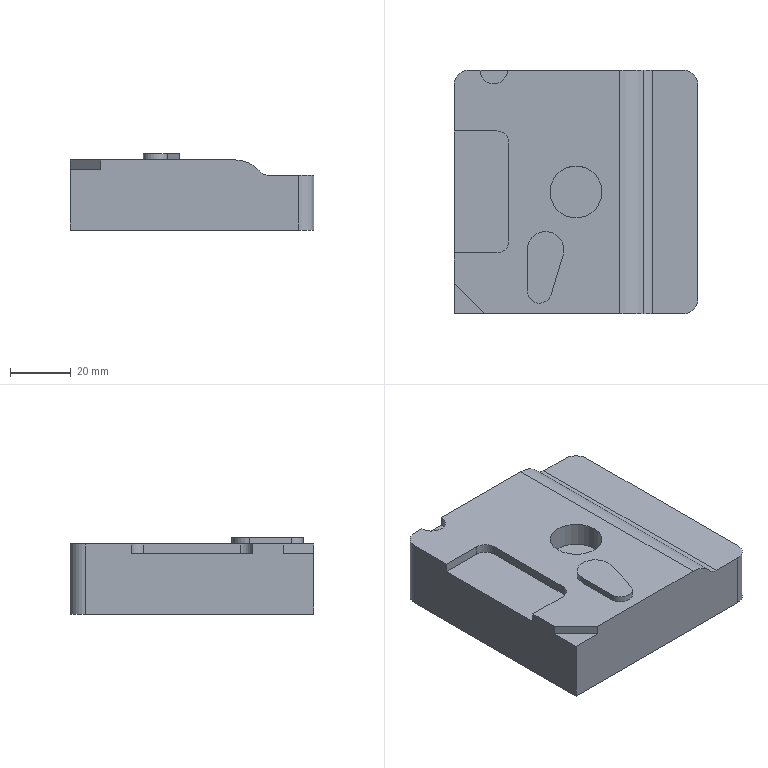NC program | NX | posted with a generic post | part box 80 x 80 x 25 mm
Lines 7698 to 8300 of 8300:
(FIXED_CONTOUR , TOOL : B6)
N15382 M6
N15384 G53
N15386 G17 G0 G90 X25.063 Y43.002 S0 M3
N15388 G43 Z8. H0
N15390 Z-1.995
N15392 G94 G1 Y42.899 Z-2.772 F250.
N15394 Y42.6 Z-3.495
N15396 Y42.123 Z-4.117
N15398 Y41.502 Z-4.594
N15400 Y40.778 Z-4.893
N15402 Y40.002 Z-4.995
N15404 Y38.203
N15406 Y36.403
N15408 Y34.603
N15410 Y32.803
N15412 Y31.003
N15414 Y29.203
N15416 Y27.403
N15418 Y25.603
N15420 Y23.803
N15422 Y22.003
N15424 Y20.203
N15426 Y18.403
N15428 Y16.603
N15430 X25.062 Y14.803
N15432 Y13.003
N15434 Y11.203
N15436 Y9.403
N15438 Y7.603
N15440 Y5.803
N15442 Y4.003
N15444 Y2.203
N15446 Y0.403
N15448 Y-1.397
N15450 Y-3.197
N15452 Y-4.997
N15454 Y-6.797
N15456 Y-8.597
N15458 Y-10.397
N15460 Y-12.197
N15462 Y-13.997
N15464 Y-15.797
N15466 Y-17.597
N15468 Y-19.397
N15470 Y-21.197
N15472 Y-22.997
N15474 Y-24.797
N15476 Y-26.597
N15478 Y-28.397
N15480 Y-30.197
N15482 Y-31.997
N15484 Y-33.797
N15486 Y-35.597
N15488 Y-37.397
N15490 Y-39.197
N15492 Y-40.06 Z-4.996
N15494 X25.026 Y-39.998 Z-4.993
N15496 X24.902 Z-4.981
N15498 X24.736 Z-4.94
N15500 X24.405 Z-4.744
N15502 X24.163 Z-4.49
N15504 Y-39.197
N15506 Y-37.397
N15508 Y-35.597
N15510 Y-33.797
N15512 Y-31.997
N15514 Y-30.197 Z-4.491
N15516 Y-28.397
N15518 Y-26.597
N15520 Y-24.797
N15522 Y-22.997
N15524 Y-21.197
N15526 Y-19.397
N15528 Y-17.597
N15530 Y-15.797
N15532 Y-13.997
N15534 Y-12.197
N15536 Y-10.397
N15538 Y-8.597
N15540 Y-6.797
N15542 Y-4.997
N15544 Y-3.197
N15546 Y-1.397
N15548 Y0.403
N15550 Y2.203
N15552 Y4.003
N15554 Y5.803
N15556 Y7.603
N15558 Y9.403
N15560 Y11.203
N15562 Y13.003
N15564 Y14.803
N15566 X24.164 Y16.603
N15568 Y18.403
N15570 Y20.203
N15572 Y22.003
N15574 Y23.803
N15576 Y25.603
N15578 Y27.403
N15580 Y29.203
N15582 Y31.003
N15584 Y32.803
N15586 Y34.603
N15588 Y36.403
N15590 Y38.203 Z-4.492
N15592 Y39.998
N15594 X23.181 Z-3.476
N15596 Y38.203
N15598 Y36.403
N15600 Y34.603
N15602 Y32.803
N15604 Y31.003
N15606 Y29.203
N15608 Y27.403
N15610 Y25.603
N15612 Y23.803
N15614 Y22.003
N15616 Y20.203
N15618 Y18.403
N15620 Y16.603
N15622 Y14.803
N15624 Y13.003
N15626 Y11.203
N15628 Y9.403
N15630 Y7.603
N15632 Y5.803
N15634 Y4.003
N15636 Y2.203
N15638 Y0.403
N15640 Y-1.397
N15642 Y-3.197
N15644 Y-4.997
N15646 Y-6.797
N15648 Y-8.597
N15650 Y-10.397
N15652 Y-12.197
N15654 Y-13.997
N15656 Y-15.797
N15658 Y-17.597
N15660 Y-19.397
N15662 Y-21.197
N15664 Y-22.997
N15666 Y-24.797
N15668 X23.18 Y-26.597
N15670 Y-28.397
N15672 Y-30.197
N15674 Y-31.997
N15676 Y-33.797
N15678 Y-35.597
N15680 Y-37.397 Z-3.475
N15682 Y-39.197
N15684 Y-39.998
N15686 X22.198 Y-39.992 Z-2.644
N15688 Y-39.197
N15690 Y-37.397
N15692 Y-35.597
N15694 Y-33.797
N15696 Y-31.997
N15698 Y-30.197 Z-2.645
N15700 Y-28.397
N15702 Y-26.597
N15704 Y-24.797
N15706 Y-22.997
N15708 Y-21.197
N15710 Y-19.397
N15712 Y-17.597
N15714 Y-15.797
N15716 Y-13.997
N15718 Y-12.197
N15720 Y-10.397
N15722 Y-8.597
N15724 Y-6.797
N15726 Y-4.997
N15728 Y-3.197
N15730 Y-1.397
N15732 Y0.403
N15734 Y2.203
N15736 Y4.003
N15738 Y5.803
N15740 Y7.603
N15742 Y9.403
N15744 X22.199 Y11.203
N15746 Y13.003
N15748 Y14.803
N15750 Y16.603
N15752 Y18.403
N15754 Y20.203
N15756 Y22.003
N15758 Y23.803
N15760 Y25.603
N15762 Y27.403
N15764 Y29.203
N15766 Y31.003
N15768 Y32.803
N15770 Y34.603
N15772 Y36.403
N15774 Y38.203
N15776 Y39.992
N15778 X21.216 Y39.998 Z-1.974
N15780 Y38.203
N15782 Y36.403
N15784 Y34.603
N15786 Y32.803
N15788 Y31.003
N15790 Y29.203
N15792 Y27.403
N15794 Y25.603
N15796 Y23.803
N15798 Y22.003
N15800 Y20.203
N15802 Y18.403
N15804 Y16.603
N15806 Y14.803
N15808 Y13.003
N15810 Y11.203
N15812 Y9.403
N15814 Y7.603
N15816 Y5.803
N15818 Y4.003
N15820 Y2.203
N15822 Y0.403
N15824 Y-1.397
N15826 Y-3.197
N15828 Y-4.997
N15830 Y-6.797
N15832 Y-8.597
N15834 Y-10.397
N15836 Y-12.197
N15838 Y-13.997
N15840 Y-15.797
N15842 Y-17.597
N15844 Y-19.397
N15846 Y-21.197
N15848 Y-22.997
N15850 Y-24.797
N15852 Y-26.597
N15854 Y-28.397
N15856 Y-30.197
N15858 X21.215 Y-31.997
N15860 Y-33.797
N15862 Y-35.597
N15864 Y-37.397
N15866 Y-39.197
N15868 Y-39.998
N15870 X20.233 Y-39.996 Z-1.42
N15872 Y-39.197
N15874 Y-37.397
N15876 Y-35.597
N15878 Y-33.797
N15880 Y-31.997
N15882 Y-30.197
N15884 Y-28.397
N15886 Y-26.597
N15888 Y-24.797
N15890 Y-22.997
N15892 Y-21.197
N15894 Y-19.397
N15896 Y-17.597
N15898 Y-15.797
N15900 Y-13.997
N15902 Y-12.197
N15904 Y-10.397
N15906 Y-8.597
N15908 Y-6.797
N15910 Y-4.997
N15912 Y-3.197
N15914 Y-1.397
N15916 Y0.403
N15918 Y2.203
N15920 X20.234 Y4.003
N15922 Y5.803
N15924 Y7.603
N15926 Y9.403
N15928 Y11.203
N15930 Y13.003
N15932 Y14.803
N15934 Y16.603
N15936 Y18.403
N15938 Y20.203
N15940 Y22.003
N15942 Y23.803
N15944 Y25.603
N15946 Y27.403
N15948 Y29.203
N15950 Y31.003
N15952 Y32.803
N15954 Y34.603
N15956 Y36.403
N15958 Y38.203
N15960 Y39.996
N15962 X19.252 Y39.991 Z-0.97
N15964 X19.251 Y38.203
N15966 Y36.403
N15968 Y34.603
N15970 Y32.803
N15972 Y31.003
N15974 Y29.203
N15976 Y27.403
N15978 Y25.603
N15980 Y23.803 Z-0.969
N15982 Y22.003
N15984 Y20.203
N15986 Y18.403
N15988 Y16.603
N15990 Y14.803
N15992 Y13.003
N15994 Y11.203
N15996 Y9.403
N15998 Y7.603
N16000 Y5.803
N16002 Y4.003
N16004 Y2.203
N16006 Y0.403
N16008 Y-1.397
N16010 Y-3.197
N16012 Y-4.997
N16014 Y-6.797
N16016 Y-8.597
N16018 Y-10.397
N16020 Y-12.197
N16022 Y-13.997
N16024 Y-15.797
N16026 Y-17.597
N16028 Y-19.397
N16030 Y-21.197
N16032 Y-22.997
N16034 Y-24.797
N16036 Y-26.597
N16038 Y-28.397
N16040 Y-30.197
N16042 Y-31.997
N16044 Y-33.797
N16046 Y-35.597
N16048 X19.25 Y-37.397
N16050 Y-39.197
N16052 Y-39.991
N16054 X18.548 Y-39.998 Z-0.707
N16056 X18.268 Y-39.995 Z-0.612
N16058 Y-39.197
N16060 Y-37.397
N16062 Y-35.597
N16064 Y-33.797
N16066 Y-31.997
N16068 Y-30.197
N16070 Y-28.397
N16072 Y-26.597
N16074 Y-24.797
N16076 Y-22.997
N16078 Y-21.197
N16080 Y-19.397
N16082 Y-17.597
N16084 Y-15.797
N16086 Y-13.997
N16088 Y-12.197
N16090 Y-10.397
N16092 Y-8.597
N16094 Y-6.797
N16096 Y-4.997
N16098 Y-3.197
N16100 X18.269 Y-1.397
N16102 Y0.403
N16104 Y2.203
N16106 Y4.003
N16108 Y5.803
N16110 Y7.603
N16112 Y9.403
N16114 Y11.203
N16116 Y13.003
N16118 Y14.803
N16120 Y16.603
N16122 Y18.403
N16124 Y20.203
N16126 Y22.003
N16128 Y23.803
N16130 Y25.603
N16132 Y27.403
N16134 Y29.203
N16136 Y31.003
N16138 Y32.803
N16140 Y34.603
N16142 Y36.403
N16144 Y38.203
N16146 Y39.995
N16148 X17.806 Y39.991 Z-0.476
N16150 X17.287 Y39.996 Z-0.341
N16152 Y38.203
N16154 Y36.403
N16156 Y34.603
N16158 X17.286 Y32.803
N16160 Y31.003
N16162 Y29.203
N16164 Y27.403
N16166 Y25.603
N16168 Y23.803
N16170 Y22.003
N16172 Y20.203
N16174 Y18.403
N16176 Y16.603
N16178 Y14.803
N16180 Y13.003
N16182 Y11.203
N16184 Y9.403
N16186 Y7.603
N16188 Y5.803
N16190 Y4.003
N16192 Y2.203
N16194 Y0.403
N16196 Y-1.397
N16198 Y-3.197
N16200 Y-4.997
N16202 Y-6.797
N16204 Y-8.597
N16206 Y-10.397
N16208 Y-12.197
N16210 Y-13.997 Z-0.34
N16212 Y-15.797
N16214 Y-17.597
N16216 Y-19.397
N16218 Y-21.197
N16220 Y-22.997
N16222 Y-24.797
N16224 Y-26.597
N16226 Y-28.397
N16228 Y-30.197
N16230 Y-31.997
N16232 Y-33.797
N16234 Y-35.597
N16236 Y-37.397
N16238 Y-39.197
N16240 Y-39.996
N16242 X16.303 Y-39.991 Z-0.15
N16244 Y-39.197
N16246 Y-37.397
N16248 Y-35.597
N16250 Y-33.797
N16252 Y-31.997
N16254 Y-30.197
N16256 Y-28.397
N16258 Y-26.597
N16260 Y-24.797
N16262 Y-22.997
N16264 Y-21.197
N16266 Y-19.397
N16268 Y-17.597
N16270 Y-15.797
N16272 Y-13.997
N16274 Y-12.197
N16276 Y-10.397
N16278 Y-8.597
N16280 X16.304 Y-6.797
N16282 Y-4.997
N16284 Y-3.197
N16286 Y-1.397
N16288 Y0.403
N16290 Y2.203
N16292 Y4.003
N16294 Y5.803
N16296 Y7.603
N16298 Y9.403
N16300 Y11.203
N16302 Y13.003
N16304 Y14.803
N16306 Y16.603
N16308 Y18.403
N16310 Y20.203
N16312 Y22.003
N16314 Y23.803
N16316 Y25.603
N16318 Y27.403
N16320 Y29.203
N16322 Y31.003
N16324 Y32.803
N16326 Y34.603
N16328 Y36.403
N16330 Y38.203
N16332 Y39.991
N16334 X15.322 Z-0.037
N16336 Y38.203
N16338 Y36.403
N16340 Y34.603
N16342 Y32.803
N16344 Y31.003
N16346 Y29.203
N16348 Y27.403
N16350 X15.321 Y25.603
N16352 Y23.803
N16354 Y22.003
N16356 Y20.203
N16358 Y18.403
N16360 Y16.603
N16362 Y14.803
N16364 Y13.003
N16366 Y11.203
N16368 Y9.403
N16370 Y7.603
N16372 Y5.803
N16374 Y4.003
N16376 Y2.203
N16378 Y0.403
N16380 Y-1.397
N16382 Y-3.197
N16384 Y-4.997
N16386 Y-6.797
N16388 Y-8.597
N16390 Y-10.397
N16392 Y-12.197
N16394 Y-13.997
N16396 Y-15.797
N16398 Y-17.597
N16400 Y-19.397
N16402 Y-21.197
N16404 Y-22.997
N16406 Y-24.797
N16408 Y-26.597
N16410 Y-28.397
N16412 Y-30.197
N16414 Y-31.997
N16416 Y-33.797
N16418 Y-35.597
N16420 Y-37.397
N16422 Y-39.197
N16424 Y-39.998
N16426 X14.344 Y-39.989 Z0.
N16428 Y-39.197
N16430 Y-37.397
N16432 Y-35.597
N16434 Y-33.797
N16436 Y-31.997
N16438 Y-30.197
N16440 Y-28.397
N16442 Y-26.597
N16444 Y-24.797
N16446 Y-22.997
N16448 Y-21.197
N16450 Y-19.397
N16452 Y-17.597
N16454 Y-15.797
N16456 Y-13.997
N16458 Y-12.197
N16460 Y-10.397
N16462 Y-8.597
N16464 Y-6.797
N16466 Y-4.997
N16468 X14.345 Y-3.197
N16470 Y-1.397
N16472 Y0.403
N16474 Y2.203
N16476 Y4.003
N16478 Y5.803
N16480 Y7.603
N16482 Y9.403
N16484 Y11.203
N16486 Y13.003
N16488 Y14.803
N16490 Y16.603
N16492 Y18.403
N16494 Y20.203
N16496 Y22.003
N16498 Y23.803
N16500 Y25.603
N16502 Y27.403
N16504 Y29.203
N16506 Y31.003
N16508 Y32.803
N16510 Y34.603
N16512 Y36.403
N16514 Y38.203
N16516 Y39.994
N16518 Y40.77 Z0.102
N16520 Y41.494 Z0.402
N16522 Y42.115 Z0.879
N16524 Y42.592 Z1.5
N16526 Y42.892 Z2.224
N16528 Y42.994 Z3.
N16530 G0 Z8.
N16532 M5
(PLANAR_PROFILE , TOOL : D6)
N16534 M6
N16536 G53
N16538 G17 G0 G90 X-46. Y-5.5 S0 M3
N16540 G43 Z8. H0
N16542 Z-20.
N16544 G94 G1 Z-23. F250.
N16546 G3 X-43. Y-2.5 R3.
N16548 G1 Y35.
N16550 G2 X-35. Y43. R8.
N16552 G1 X35.
N16554 G2 X43. Y35. R8.
N16556 G1 Y-35.
N16558 G2 X35. Y-43. R8.
N16560 G1 X-40.
N16562 G2 X-43. Y-40. R3.
N16564 G1 Y-2.5
N16566 G3 X-46. Y0.5 R3.
N16568 G1 Z-20.
N16570 G0 Z8.
N16572 M5
N16574 M2